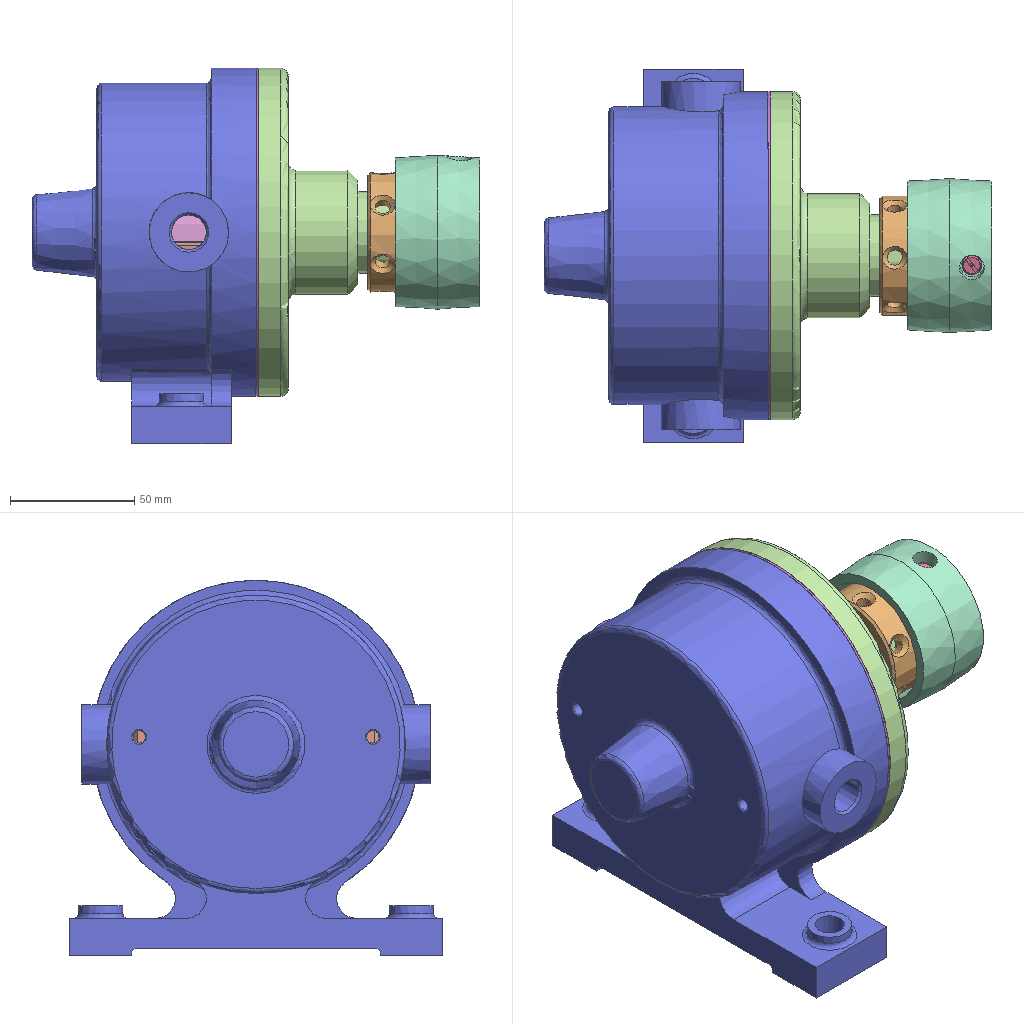Assembly | NX | 16 different items | 22 placed | box 180 x 150 x 151 mm
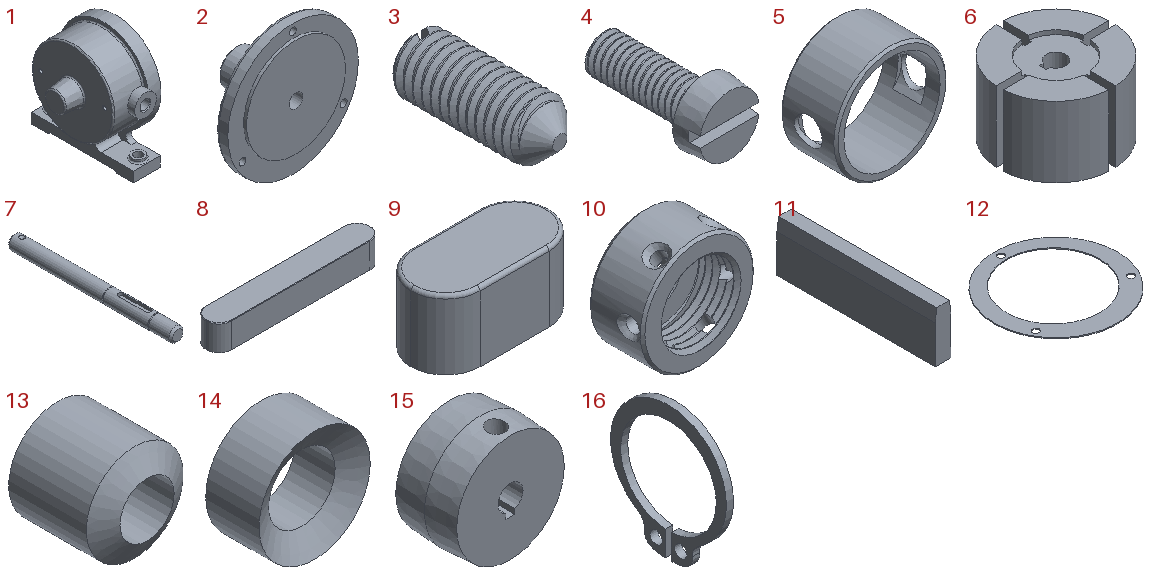Parts list (item | quantity | size | volume | features):
1 | x1 | 90 x 150 x 151 mm | 479764 mm3 | features DATUM_CSYS 16, SKETCH 15, EXTRACT_FACE 11, EXTRUDE 10, HOLE PACKAGE 7, SIMPLE HOLE 7, SYMBOLIC_THREAD 7, Instance Feature 5, BLEND 3, Mirror Feature 3, EXTRACT_DATUM_AXIS 2, EXTRACT_DATUM_PLANE 2, EXTRACT_STRING 2, DATUM_AXIS 1, DATUM_PLANE 1, Pattern Feature 1, SWP104 1, UNITE 1
2 | x1 | 132 x 61 x 132 mm | 237837 mm3 | features DATUM_CSYS 7, SKETCH 6, CBORE_HOLE 3, EXTRACT_FACE 3, EXTRUDE 3, HOLE PACKAGE 3, CHAMFER 2, Instance Feature 2, BLEND 1, Pattern Feature 1, SWP104 1
3 | x1 | 8 x 20 x 8 mm | 753.077 mm3 | features DATUM_CSYS 3, SKETCH 2, CHAMFER 1, EXTRUDE 1, SWP104 1, THREADS 1
4 | x3 | 10 x 19.9 x 10 mm | 653.386 mm3 | features DATUM_CSYS 3, SKETCH 2, EXTRUDE 1, SWP104 1, THREADS 1
5 | x1 | 100.002 x 50 x 100 mm | 93333 mm3 | features DATUM_CSYS 6, EXTRUDE 5, SKETCH 5, EXTRACT_DATUM_AXIS 4, EXTRACT_DATUM_PLANE 4, EXTRACT_STRING 4, CHAMFER 1, Instance Feature 1, Mirror Feature 1
6 | x1 | 79.844 x 79.844 x 50 mm | 215152 mm3 | features DATUM_CSYS 7, EXTRUDE 7, SKETCH 6, EXTRACT_DATUM_AXIS 4, EXTRACT_FACE 4, Instance Feature 3, Pattern Feature 1
7 | x1 | 14 x 162 x 14 mm | 24153 mm3 | features DATUM_CSYS 4, SKETCH 3, EXTRUDE 2, SWP104 2, CHAMFER 1, CYLINDER 1
8 | x1 | 32 x 5 x 5 mm | 772.96 mm3 | features BLEND 2, DATUM_CSYS 2, EXTRUDE 1, SKETCH 1
9 | x1 | 10 x 5 x 5 mm | 222.861 mm3 | features BLEND 2, DATUM_CSYS 2, EXTRUDE 1, SKETCH 1
10 | x1 | 48 x 24 x 48 mm | 25018 mm3 | features DATUM_CSYS 8, SKETCH 7, SWP104 7, EXTRACT_DATUM_AXIS 6, EXTRACT_DATUM_PLANE 6, EXTRACT_FACE 6, Instance Feature 5, CHAMFER 2, DATUM_PLANE 1, Pattern Feature 1, THREADS 1
11 | x4 | 5 x 50 x 16 mm | 3900 mm3 | features DATUM_CSYS 2, EXTRUDE 1, SKETCH 1
12 | x1 | 132 x 132 x 1 mm | 5715 mm3 | features DATUM_CSYS 2, EXTRUDE 1, SKETCH 1
13 | x1 | 25 x 26.35 x 25 mm | 7708 mm3 | features DATUM_CSYS 4, SKETCH 3, EXTRACT_DATUM_AXIS 2, EXTRACT_DATUM_PLANE 2, EXTRACT_FACE 2, EXTRACT_STRING 2, SWP104 2, EXTRUDE 1, Instance Feature 1, Mirror Feature 1
14 | x1 | 25 x 12 x 25 mm | 3354 mm3 | features DATUM_CSYS 2, SKETCH 1, SWP104 1
15 | x1 | 62 x 34 x 62 mm | 57319 mm3 | features DATUM_CSYS 6, SKETCH 5, HOLE PACKAGE 2, SIMPLE HOLE 2, SWP104 2, EXTRUDE 1, SYMBOLIC_THREAD 1
16 | x2 | 1 x 16.22 x 18.771 mm | 75.444 mm3 | features DATUM_CSYS 2, EXTRUDE 1, SKETCH 1
Mates (type | each side: item.copy, entity, surface, feature):
Fix | 1.1 component
Touch | 8.1 face plane Extrude(1) | 7.1 face plane Extrude(6) | 2 times
Touch | 5.1 face cylinder Extrude(1) | 1.1 face cylinder Revolve(9)
Touch | 5.1 face plane Extrude(1) | 1.1 face plane Revolve(9)
Touch | 2.1 face cylinder Revolve(4) | 5.1 face cylinder Extrude(1) | 2 times
Touch | 2.1 face cylinder Ø7 Counterbored Hole(9) | 1.1 face cylinder M6 x 1.0 Threaded Hole(14)
Angle | 5.1 face cylinder Extrude(4) | 1.1 face cylinder M16 x 2 Threaded Hole(24)
Touch | 12.1 face cylinder Extrude(1) | 1.1 face cylinder M6 x 1.0 Threaded Hole(14)
Touch | 12.1 face cylinder Extrude(1) | 1.1 face cylinder Pattern Feature [Circular] (16) / Instance[2][0]
Touch | 12.1 face plane Extrude(1) | 1.1 face plane Revolve(9)
Touch | 2.1 face plane Extrude(3) | 12.1 face plane Extrude(1)
Touch | 3.1 face cylinder Threads(3) | 7.1 face cone Revolve(4)
Touch | 3.1 face cone Revolve(1) | 7.1 face cone Revolve(4)
Touch | 7.1 face cylinder Cylinder(1) | 15.1 face cylinder Extrude(3)
Touch | 3.1 face cylinder Revolve(1) | 15.1 face cylinder Revolve(4)
Touch | 8.1 face cylinder Edge Blend(2) | 7.1 face cylinder Extrude(6)
Touch | 10.1 face cylinder Revolve(1) | 7.1 face cylinder Cylinder(1)
Touch | 13.1 face cylinder Extrude(1) | 7.1 face cylinder Cylinder(1)
Touch | 6.1 face cylinder Extrude(1) | 7.1 face cylinder Cylinder(1)
Touch | 6.1 face plane Extrude(3) | 8.1 face plane Extrude(1)
Touch | 16.1 face cylinder Extrude(1) | 7.1 face cylinder Cylinder(1) | 2 times
Touch | 16.1 face plane Extrude(1) | 7.1 face plane Revolve(3)
Touch | 6.1 face plane Extrude(2) | 16.1 face plane Extrude(1)
Touch | 16.1 face plane Extrude(1) | 6.1 face plane Extrude(2)
Touch | 7.1 face cylinder Cylinder(1) | 5.1 face cylinder Extrude(1)
Touch | 14.1 face cylinder Revolve(1) | 7.1 face cylinder Cylinder(1)
Touch | 13.1 face cone Mirror Feature(3) | 14.1 face cone Revolve(1)
Touch | 11.1 face plane Extrude(1) | 6.1 face plane Pattern Feature [Circular] (5) / Instance[1][0]
Touch | 4.1 face cone Revolve(1) | 2.1 face cylinder Ø7 Counterbored Hole(9)
Touch | 4.1 face plane Revolve(1) | 2.1 face plane Ø7 Counterbored Hole(9)
Touch | 4.1 face cone Revolve(1) | 2.1 face cylinder Pattern Feature [Circular] (10) / Instance[1][0]
Touch | 4.1 face plane Revolve(1) | 2.1 face plane Pattern Feature [Circular] (10) / Instance[1][0]
Touch | 4.1 face cone Revolve(1) | 2.1 face cylinder Pattern Feature [Circular] (10) / Instance[2][0]
Touch | 4.1 face plane Revolve(1) | 2.1 face plane Pattern Feature [Circular] (10) / Instance[2][0]
Touch | 9.1 face plane Extrude(1) | 7.1 face plane Extrude(7) | 2 times
Touch | 9.1 face cylinder Edge Blend(2) | 7.1 face cylinder Extrude(7)
Touch | 13.1 face cone Revolve(2) | 2.1 face cone Revolve(4)
Touch | 6.1 face plane Extrude(1) | 1.1 face plane Revolve(9)
Distance | 10.1 face plane Revolve(1) | 15.1 face plane Ø52 Hole(2)
Touch | 11.1 face plane Extrude(1) | 6.1 face plane Extrude(1)
Distance | 11.1 face plane Extrude(1) | 6.1 face plane Pattern Feature [Circular] (5) / Instance[1][0]
Bond | 7.1 component | assembly component
Bond | 11.1 component | assembly component | 4 times
CircularPattern | assembly axis | assembly csys | assembly csys | assembly csys | assembly csys